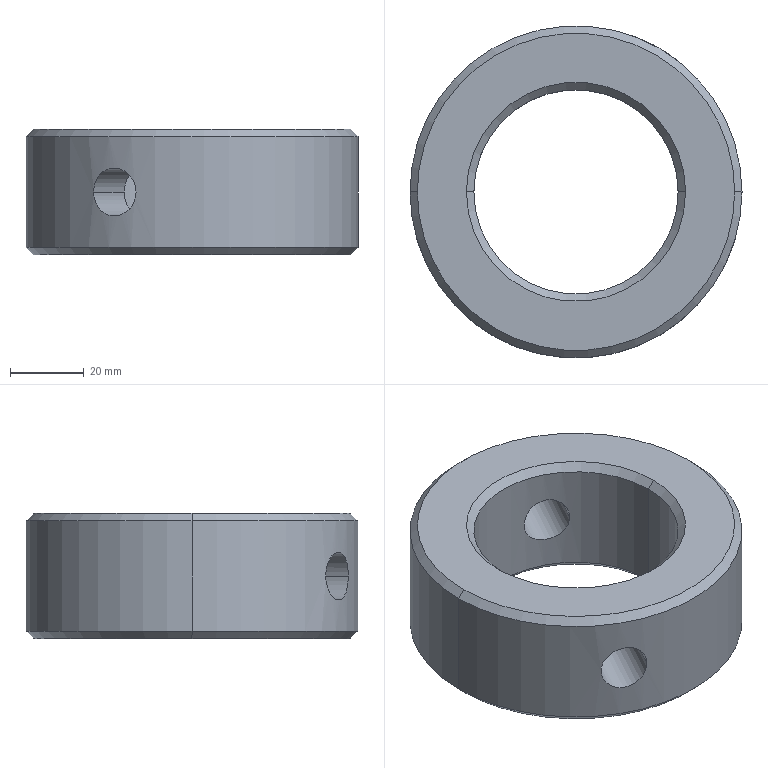Part | SolidWorks | features 3DProfileFeature 1, Chamfer 1, Extrusion 1, HoleWzd 1 | 1 solid | 18 faces | box 90 x 90 x 34 mm | volume 127902 mm3 | cone 8 | cylinder 8 | plane 2 | commonest cylinder face diameters 13 x4 55.4 x2 90 x2
STEP:
#1=CARTESIAN_POINT('',(43.,0.,34.));
#2=VERTEX_POINT('',#1);
#3=CARTESIAN_POINT('',(-43.,0.,34.));
#4=VERTEX_POINT('',#3);
#5=CARTESIAN_POINT('',(0.,0.,34.));
#6=DIRECTION('',(0.,0.,1.));
#7=DIRECTION('',(1.,0.,0.));
#8=AXIS2_PLACEMENT_3D('',#5,#6,#7);
#9=CIRCLE('',#8,43.);
#10=EDGE_CURVE('',#2,#4,#9,.T.);
#11=ORIENTED_EDGE('',*,*,#10,.F.);
#12=CARTESIAN_POINT('',(45.,0.,32.));
#13=VERTEX_POINT('',#12);
#14=CARTESIAN_POINT('',(43.,0.,34.));
#15=DIRECTION('',(0.7071,0.,-0.7071));
#16=VECTOR('',#15,1000.);
#17=LINE('',#14,#16);
#18=EDGE_CURVE('',#2,#13,#17,.T.);
#19=ORIENTED_EDGE('',*,*,#18,.T.);
#20=CARTESIAN_POINT('',(-45.,0.,32.));
#21=VERTEX_POINT('',#20);
#22=CARTESIAN_POINT('',(0.,0.,32.));
#23=DIRECTION('',(0.,0.,-1.));
#24=DIRECTION('',(1.,0.,0.));
#25=AXIS2_PLACEMENT_3D('',#22,#23,#24);
#26=CIRCLE('',#25,45.);
#27=EDGE_CURVE('',#21,#13,#26,.T.);
#28=ORIENTED_EDGE('',*,*,#27,.F.);
#29=CARTESIAN_POINT('',(-43.,0.,34.));
#30=DIRECTION('',(-0.7071,0.,-0.7071));
#31=VECTOR('',#30,1000.);
#32=LINE('',#29,#31);
#33=EDGE_CURVE('',#4,#21,#32,.T.);
#34=ORIENTED_EDGE('',*,*,#33,.F.);
#35=EDGE_LOOP('',(#11,#19,#28,#34));
#36=FACE_OUTER_BOUND('',#35,.T.);
#37=CARTESIAN_POINT('',(0.,0.,34.));
#38=DIRECTION('',(0.,0.,-1.));
#39=DIRECTION('',(-1.,0.,0.));
#40=AXIS2_PLACEMENT_3D('',#37,#38,#39);
#41=CONICAL_SURFACE('',#40,43.,0.7854);
#42=ADVANCED_FACE('',(#36),#41,.T.);
#43=CARTESIAN_POINT('',(-27.7,0.,32.));
#44=VERTEX_POINT('',#43);
#45=CARTESIAN_POINT('',(27.7,0.,32.));
#46=VERTEX_POINT('',#45);
#47=CARTESIAN_POINT('',(0.,0.,32.));
#48=DIRECTION('',(0.,0.,1.));
#49=DIRECTION('',(1.,0.,0.));
#50=AXIS2_PLACEMENT_3D('',#47,#48,#49);
#51=CIRCLE('',#50,27.7);
#52=EDGE_CURVE('',#44,#46,#51,.T.);
#53=ORIENTED_EDGE('',*,*,#52,.F.);
#54=CARTESIAN_POINT('',(-29.7,0.,34.));
#55=VERTEX_POINT('',#54);
#56=CARTESIAN_POINT('',(-27.7,0.,32.));
#57=DIRECTION('',(-0.7071,0.,0.7071));
#58=VECTOR('',#57,1000.);
#59=LINE('',#56,#58);
#60=EDGE_CURVE('',#44,#55,#59,.T.);
#61=ORIENTED_EDGE('',*,*,#60,.T.);
#62=CARTESIAN_POINT('',(29.7,0.,34.));
#63=VERTEX_POINT('',#62);
#64=CARTESIAN_POINT('',(0.,0.,34.));
#65=DIRECTION('',(0.,0.,-1.));
#66=DIRECTION('',(1.,0.,0.));
#67=AXIS2_PLACEMENT_3D('',#64,#65,#66);
#68=CIRCLE('',#67,29.7);
#69=EDGE_CURVE('',#63,#55,#68,.T.);
#70=ORIENTED_EDGE('',*,*,#69,.F.);
#71=CARTESIAN_POINT('',(27.7,0.,32.));
#72=DIRECTION('',(0.7071,0.,0.7071));
#73=VECTOR('',#72,1000.);
#74=LINE('',#71,#73);
#75=EDGE_CURVE('',#46,#63,#74,.T.);
#76=ORIENTED_EDGE('',*,*,#75,.F.);
#77=EDGE_LOOP('',(#53,#61,#70,#76));
#78=FACE_OUTER_BOUND('',#77,.T.);
#79=CARTESIAN_POINT('',(0.,0.,32.));
#80=DIRECTION('',(0.,0.,1.));
#81=DIRECTION('',(1.,0.,0.));
#82=AXIS2_PLACEMENT_3D('',#79,#80,#81);
#83=CONICAL_SURFACE('',#82,27.7,0.7854);
#84=ADVANCED_FACE('',(#78),#83,.F.);
#85=CARTESIAN_POINT('',(27.7,0.,2.));
#86=VERTEX_POINT('',#85);
#87=CARTESIAN_POINT('',(-27.7,0.,2.));
#88=VERTEX_POINT('',#87);
#89=CARTESIAN_POINT('',(0.,0.,2.));
#90=DIRECTION('',(0.,0.,-1.));
#91=DIRECTION('',(1.,0.,0.));
#92=AXIS2_PLACEMENT_3D('',#89,#90,#91);
#93=CIRCLE('',#92,27.7);
#94=EDGE_CURVE('',#86,#88,#93,.T.);
#95=ORIENTED_EDGE('',*,*,#94,.F.);
#96=CARTESIAN_POINT('',(29.7,0.,0.));
#97=VERTEX_POINT('',#96);
#98=CARTESIAN_POINT('',(29.7,0.,0.));
#99=DIRECTION('',(0.7071,0.,-0.7071));
#100=VECTOR('',#99,1000.);
#101=LINE('',#98,#100);
#102=EDGE_CURVE('',#86,#97,#101,.T.);
#103=ORIENTED_EDGE('',*,*,#102,.T.);
#104=CARTESIAN_POINT('',(-29.7,0.,0.));
#105=VERTEX_POINT('',#104);
#106=CARTESIAN_POINT('',(0.,0.,0.));
#107=DIRECTION('',(0.,0.,1.));
#108=DIRECTION('',(1.,0.,0.));
#109=AXIS2_PLACEMENT_3D('',#106,#107,#108);
#110=CIRCLE('',#109,29.7);
#111=EDGE_CURVE('',#105,#97,#110,.T.);
#112=ORIENTED_EDGE('',*,*,#111,.F.);
#113=CARTESIAN_POINT('',(-29.7,0.,0.));
#114=DIRECTION('',(-0.7071,0.,-0.7071));
#115=VECTOR('',#114,1000.);
#116=LINE('',#113,#115);
#117=EDGE_CURVE('',#88,#105,#116,.T.);
#118=ORIENTED_EDGE('',*,*,#117,.F.);
#119=EDGE_LOOP('',(#95,#103,#112,#118));
#120=FACE_OUTER_BOUND('',#119,.T.);
#121=CARTESIAN_POINT('',(0.,0.,0.));
#122=DIRECTION('',(0.,0.,-1.));
#123=DIRECTION('',(-1.,0.,0.));
#124=AXIS2_PLACEMENT_3D('',#121,#122,#123);
#125=CONICAL_SURFACE('',#124,29.7,0.7854);
#126=ADVANCED_FACE('',(#120),#125,.F.);
#127=CARTESIAN_POINT('',(-43.,0.,0.));
#128=VERTEX_POINT('',#127);
#129=CARTESIAN_POINT('',(43.,0.,0.));
#130=VERTEX_POINT('',#129);
#131=CARTESIAN_POINT('',(0.,0.,0.));
#132=DIRECTION('',(0.,0.,-1.));
#133=DIRECTION('',(1.,0.,0.));
#134=AXIS2_PLACEMENT_3D('',#131,#132,#133);
#135=CIRCLE('',#134,43.);
#136=EDGE_CURVE('',#128,#130,#135,.T.);
#137=ORIENTED_EDGE('',*,*,#136,.F.);
#138=CARTESIAN_POINT('',(-45.,0.,2.));
#139=VERTEX_POINT('',#138);
#140=CARTESIAN_POINT('',(-45.,0.,2.));
#141=DIRECTION('',(-0.7071,0.,0.7071));
#142=VECTOR('',#141,1000.);
#143=LINE('',#140,#142);
#144=EDGE_CURVE('',#128,#139,#143,.T.);
#145=ORIENTED_EDGE('',*,*,#144,.T.);
#146=CARTESIAN_POINT('',(45.,0.,2.));
#147=VERTEX_POINT('',#146);
#148=CARTESIAN_POINT('',(0.,0.,2.));
#149=DIRECTION('',(0.,0.,1.));
#150=DIRECTION('',(1.,0.,0.));
#151=AXIS2_PLACEMENT_3D('',#148,#149,#150);
#152=CIRCLE('',#151,45.);
#153=EDGE_CURVE('',#147,#139,#152,.T.);
#154=ORIENTED_EDGE('',*,*,#153,.F.);
#155=CARTESIAN_POINT('',(45.,0.,2.));
#156=DIRECTION('',(0.7071,0.,0.7071));
#157=VECTOR('',#156,1000.);
#158=LINE('',#155,#157);
#159=EDGE_CURVE('',#130,#147,#158,.T.);
#160=ORIENTED_EDGE('',*,*,#159,.F.);
#161=EDGE_LOOP('',(#137,#145,#154,#160));
#162=FACE_OUTER_BOUND('',#161,.T.);
#163=CARTESIAN_POINT('',(0.,0.,2.));
#164=DIRECTION('',(0.,0.,1.));
#165=DIRECTION('',(1.,0.,0.));
#166=AXIS2_PLACEMENT_3D('',#163,#164,#165);
#167=CONICAL_SURFACE('',#166,45.,0.7854);
#168=ADVANCED_FACE('',(#162),#167,.T.);
#169=CARTESIAN_POINT('',(-15.171,-42.366,17.));
#170=VERTEX_POINT('',#169);
#171=CARTESIAN_POINT('',(-26.648,-36.261,17.));
#172=VERTEX_POINT('',#171);
#173=CARTESIAN_POINT('',(-15.171,-42.366,17.));
#174=CARTESIAN_POINT('',(-15.171,-42.366,16.576));
#175=CARTESIAN_POINT('',(-15.21,-42.352,16.153));
#176=CARTESIAN_POINT('',(-15.329,-42.309,15.523));
#177=CARTESIAN_POINT('',(-15.378,-42.291,15.315));
#178=CARTESIAN_POINT('',(-15.496,-42.248,14.908));
#179=CARTESIAN_POINT('',(-15.631,-42.198,14.509));
#180=CARTESIAN_POINT('',(-15.802,-42.134,14.126));
#181=CARTESIAN_POINT('',(-15.991,-42.063,13.75));
#182=CARTESIAN_POINT('',(-16.095,-42.023,13.566));
#183=CARTESIAN_POINT('',(-16.43,-41.894,13.034));
#184=CARTESIAN_POINT('',(-16.681,-41.795,12.707));
#185=CARTESIAN_POINT('',(-17.239,-41.568,12.107));
#186=CARTESIAN_POINT('',(-17.548,-41.439,11.833));
#187=CARTESIAN_POINT('',(-18.197,-41.158,11.361));
#188=CARTESIAN_POINT('',(-18.539,-41.006,11.161));
#189=CARTESIAN_POINT('',(-19.075,-40.758,10.916));
#190=CARTESIAN_POINT('',(-19.259,-40.671,10.843));
#191=CARTESIAN_POINT('',(-19.627,-40.495,10.719));
#192=CARTESIAN_POINT('',(-19.813,-40.404,10.667));
#193=CARTESIAN_POINT('',(-20.371,-40.127,10.543));
#194=CARTESIAN_POINT('',(-20.748,-39.934,10.5));
#195=CARTESIAN_POINT('',(-21.507,-39.53,10.5));
#196=CARTESIAN_POINT('',(-21.877,-39.327,10.542));
#197=CARTESIAN_POINT('',(-22.419,-39.018,10.665));
#198=CARTESIAN_POINT('',(-22.598,-38.915,10.717));
#199=CARTESIAN_POINT('',(-22.951,-38.708,10.84));
#200=CARTESIAN_POINT('',(-23.125,-38.604,10.913));
#201=CARTESIAN_POINT('',(-23.631,-38.298,11.157));
#202=CARTESIAN_POINT('',(-23.948,-38.1,11.357));
#203=CARTESIAN_POINT('',(-24.546,-37.718,11.828));
#204=CARTESIAN_POINT('',(-24.826,-37.533,12.102));
#205=CARTESIAN_POINT('',(-25.326,-37.198,12.7));
#206=CARTESIAN_POINT('',(-25.549,-37.045,13.026));
#207=CARTESIAN_POINT('',(-25.942,-36.77,13.737));
#208=CARTESIAN_POINT('',(-26.108,-36.652,14.113));
#209=CARTESIAN_POINT('',(-26.308,-36.509,14.7));
#210=CARTESIAN_POINT('',(-26.367,-36.467,14.899));
#211=CARTESIAN_POINT('',(-26.468,-36.393,15.306));
#212=CARTESIAN_POINT('',(-26.511,-36.362,15.515));
#213=CARTESIAN_POINT('',(-26.614,-36.286,16.145));
#214=CARTESIAN_POINT('',(-26.648,-36.261,16.57));
#215=CARTESIAN_POINT('',(-26.648,-36.261,17.));
#216=B_SPLINE_CURVE_WITH_KNOTS('',3,(#173,#174,#175,#176,#177,#178,#179,#180,#181,#182,#183,#184,#185,#186,#187,#188,#189,#190,#191,#192,#193,#194,#195,#196,#197,#198,#199,#200,#201,#202,#203,#204,#205,#206,#207,#208,#209,#210,#211,#212,#213,#214,#215),.UNSPECIFIED.,.F.,.F.,(4,2,2,1,2,2,2,2,2,2,2,2,2,2,2,2,2,2,2,2,2,4),(0.02035,0.02162,0.02226,0.02289,0.02353,0.02416,0.02543,0.02671,0.02798,0.02861,0.02925,0.03052,0.03179,0.03243,0.03306,0.03433,0.03561,0.03688,0.03815,0.03878,0.03942,0.04069),.UNSPECIFIED.);
#217=EDGE_CURVE('',#170,#172,#216,.T.);
#218=ORIENTED_EDGE('',*,*,#217,.F.);
#219=CARTESIAN_POINT('',(-6.905,-26.825,17.));
#220=VERTEX_POINT('',#219);
#221=CARTESIAN_POINT('',(26.87,36.678,17.));
#222=DIRECTION('',(0.4696,0.8829,0.));
#223=VECTOR('',#222,1000.);
#224=LINE('',#221,#223);
#225=EDGE_CURVE('',#170,#220,#224,.T.);
#226=ORIENTED_EDGE('',*,*,#225,.T.);
#227=CARTESIAN_POINT('',(-18.383,-20.721,17.));
#228=VERTEX_POINT('',#227);
#229=CARTESIAN_POINT('',(-6.905,-26.825,17.));
#230=CARTESIAN_POINT('',(-6.905,-26.825,16.575));
#231=CARTESIAN_POINT('',(-6.947,-26.815,16.152));
#232=CARTESIAN_POINT('',(-7.114,-26.771,15.308));
#233=CARTESIAN_POINT('',(-7.237,-26.738,14.901));
#234=CARTESIAN_POINT('',(-7.477,-26.672,14.314));
#235=CARTESIAN_POINT('',(-7.567,-26.647,14.122));
#236=CARTESIAN_POINT('',(-7.764,-26.59,13.746));
#237=CARTESIAN_POINT('',(-7.873,-26.558,13.562));
#238=CARTESIAN_POINT('',(-8.219,-26.454,13.032));
#239=CARTESIAN_POINT('',(-8.479,-26.372,12.706));
#240=CARTESIAN_POINT('',(-9.055,-26.18,12.106));
#241=CARTESIAN_POINT('',(-9.373,-26.069,11.833));
#242=CARTESIAN_POINT('',(-10.036,-25.82,11.363));
#243=CARTESIAN_POINT('',(-10.385,-25.683,11.163));
#244=CARTESIAN_POINT('',(-10.933,-25.452,10.916));
#245=CARTESIAN_POINT('',(-11.12,-25.371,10.844));
#246=CARTESIAN_POINT('',(-11.492,-25.204,10.72));
#247=CARTESIAN_POINT('',(-11.867,-25.032,10.616));
#248=CARTESIAN_POINT('',(-12.245,-24.848,10.553));
#249=CARTESIAN_POINT('',(-12.624,-24.657,10.511));
#250=CARTESIAN_POINT('',(-12.816,-24.558,10.5));
#251=CARTESIAN_POINT('',(-13.384,-24.256,10.5));
#252=CARTESIAN_POINT('',(-13.753,-24.049,10.542));
#253=CARTESIAN_POINT('',(-14.471,-23.623,10.707));
#254=CARTESIAN_POINT('',(-14.824,-23.403,10.833));
#255=CARTESIAN_POINT('',(-15.483,-22.972,11.159));
#256=CARTESIAN_POINT('',(-15.793,-22.76,11.358));
#257=CARTESIAN_POINT('',(-16.229,-22.448,11.713));
#258=CARTESIAN_POINT('',(-16.37,-22.346,11.841));
#259=CARTESIAN_POINT('',(-16.637,-22.148,12.11));
#260=CARTESIAN_POINT('',(-16.763,-22.053,12.252));
#261=CARTESIAN_POINT('',(-17.123,-21.776,12.7));
#262=CARTESIAN_POINT('',(-17.338,-21.604,13.028));
#263=CARTESIAN_POINT('',(-17.713,-21.297,13.738));
#264=CARTESIAN_POINT('',(-17.87,-21.166,14.111));
#265=CARTESIAN_POINT('',(-18.06,-21.003,14.697));
#266=CARTESIAN_POINT('',(-18.116,-20.955,14.897));
#267=CARTESIAN_POINT('',(-18.213,-20.871,15.307));
#268=CARTESIAN_POINT('',(-18.253,-20.835,15.516));
#269=CARTESIAN_POINT('',(-18.35,-20.75,16.144));
#270=CARTESIAN_POINT('',(-18.383,-20.721,16.569));
#271=CARTESIAN_POINT('',(-18.383,-20.721,17.));
#272=B_SPLINE_CURVE_WITH_KNOTS('',3,(#229,#230,#231,#232,#233,#234,#235,#236,#237,#238,#239,#240,#241,#242,#243,#244,#245,#246,#247,#248,#249,#250,#251,#252,#253,#254,#255,#256,#257,#258,#259,#260,#261,#262,#263,#264,#265,#266,#267,#268,#269,#270,#271),.UNSPECIFIED.,.F.,.F.,(4,2,2,2,2,2,2,2,2,1,2,2,2,2,2,2,2,2,2,2,2,4),(0.02039,0.02167,0.02294,0.02358,0.02422,0.02549,0.02676,0.02804,0.02868,0.02931,0.02995,0.03059,0.03186,0.03314,0.03441,0.03505,0.03568,0.03696,0.03823,0.03887,0.03951,0.04078),.UNSPECIFIED.);
#273=EDGE_CURVE('',#220,#228,#272,.T.);
#274=ORIENTED_EDGE('',*,*,#273,.T.);
#275=CARTESIAN_POINT('',(15.392,42.782,17.));
#276=DIRECTION('',(0.4696,0.8829,0.));
#277=VECTOR('',#276,1000.);
#278=LINE('',#275,#277);
#279=EDGE_CURVE('',#172,#228,#278,.T.);
#280=ORIENTED_EDGE('',*,*,#279,.F.);
#281=EDGE_LOOP('',(#218,#226,#274,#280));
#282=FACE_OUTER_BOUND('',#281,.T.);
#283=CARTESIAN_POINT('',(21.131,39.73,17.));
#284=DIRECTION('',(0.4696,0.8829,0.));
#285=DIRECTION('',(-0.8829,0.4696,0.));
#286=AXIS2_PLACEMENT_3D('',#283,#284,#285);
#287=CYLINDRICAL_SURFACE('',#286,6.5);
#288=ADVANCED_FACE('',(#282),#287,.F.);
#289=CARTESIAN_POINT('',(6.905,26.825,17.));
#290=VERTEX_POINT('',#289);
#291=CARTESIAN_POINT('',(18.383,20.721,17.));
#292=VERTEX_POINT('',#291);
#293=CARTESIAN_POINT('',(6.905,26.825,17.));
#294=CARTESIAN_POINT('',(6.905,26.825,16.569));
#295=CARTESIAN_POINT('',(6.948,26.815,16.145));
#296=CARTESIAN_POINT('',(7.072,26.782,15.521));
#297=CARTESIAN_POINT('',(7.123,26.769,15.314));
#298=CARTESIAN_POINT('',(7.246,26.736,14.905));
#299=CARTESIAN_POINT('',(7.318,26.716,14.702));
#300=CARTESIAN_POINT('',(7.56,26.649,14.112));
#301=CARTESIAN_POINT('',(7.757,26.593,13.74));
#302=CARTESIAN_POINT('',(8.102,26.489,13.211));
#303=CARTESIAN_POINT('',(8.226,26.451,13.038));
#304=CARTESIAN_POINT('',(8.489,26.368,12.709));
#305=CARTESIAN_POINT('',(8.626,26.323,12.552));
#306=CARTESIAN_POINT('',(9.057,26.179,12.104));
#307=CARTESIAN_POINT('',(9.369,26.07,11.836));
#308=CARTESIAN_POINT('',(10.04,25.819,11.36));
#309=CARTESIAN_POINT('',(10.392,25.68,11.159));
#310=CARTESIAN_POINT('',(10.934,25.451,10.916));
#311=CARTESIAN_POINT('',(11.118,25.372,10.844));
#312=CARTESIAN_POINT('',(11.491,25.205,10.72));
#313=CARTESIAN_POINT('',(11.682,25.117,10.667));
#314=CARTESIAN_POINT('',(12.251,24.847,10.542));
#315=CARTESIAN_POINT('',(12.629,24.657,10.5));
#316=CARTESIAN_POINT('',(13.381,24.257,10.5));
#317=CARTESIAN_POINT('',(13.758,24.045,10.542));
#318=CARTESIAN_POINT('',(14.477,23.619,10.709));
#319=CARTESIAN_POINT('',(14.822,23.404,10.833));
#320=CARTESIAN_POINT('',(15.32,23.079,11.078));
#321=CARTESIAN_POINT('',(15.482,22.97,11.17));
#322=CARTESIAN_POINT('',(15.794,22.757,11.371));
#323=CARTESIAN_POINT('',(15.943,22.652,11.48));
#324=CARTESIAN_POINT('',(16.232,22.447,11.715));
#325=CARTESIAN_POINT('',(16.37,22.346,11.841));
#326=CARTESIAN_POINT('',(16.637,22.148,12.11));
#327=CARTESIAN_POINT('',(16.765,22.051,12.254));
#328=CARTESIAN_POINT('',(17.128,21.772,12.706));
#329=CARTESIAN_POINT('',(17.341,21.602,13.033));
#330=CARTESIAN_POINT('',(17.712,21.298,13.736));
#331=CARTESIAN_POINT('',(17.872,21.164,14.117));
#332=CARTESIAN_POINT('',(18.126,20.947,14.902));
#333=CARTESIAN_POINT('',(18.221,20.864,15.307));
#334=CARTESIAN_POINT('',(18.318,20.778,15.934));
#335=CARTESIAN_POINT('',(18.343,20.757,16.148));
#336=CARTESIAN_POINT('',(18.375,20.728,16.575));
#337=CARTESIAN_POINT('',(18.383,20.721,16.787));
#338=CARTESIAN_POINT('',(18.383,20.721,17.));
#339=B_SPLINE_CURVE_WITH_KNOTS('',3,(#293,#294,#295,#296,#297,#298,#299,#300,#301,#302,#303,#304,#305,#306,#307,#308,#309,#310,#311,#312,#313,#314,#315,#316,#317,#318,#319,#320,#321,#322,#323,#324,#325,#326,#327,#328,#329,#330,#331,#332,#333,#334,#335,#336,#337,#338),.UNSPECIFIED.,.F.,.F.,(4,2,2,2,2,2,2,2,2,2,2,2,2,2,2,2,2,2,2,2,2,2,4),(0.,0.001275,0.001912,0.002549,0.003824,0.004461,0.005098,0.006373,0.007647,0.008285,0.008922,0.0102,0.01147,0.01275,0.01338,0.01402,0.01466,0.01529,0.01657,0.01784,0.01912,0.01976,0.02039),.UNSPECIFIED.);
#340=EDGE_CURVE('',#290,#292,#339,.T.);
#341=ORIENTED_EDGE('',*,*,#340,.T.);
#342=CARTESIAN_POINT('',(26.648,36.261,17.));
#343=VERTEX_POINT('',#342);
#344=CARTESIAN_POINT('',(26.87,36.678,17.));
#345=DIRECTION('',(0.4696,0.8829,0.));
#346=VECTOR('',#345,1000.);
#347=LINE('',#344,#346);
#348=EDGE_CURVE('',#292,#343,#347,.T.);
#349=ORIENTED_EDGE('',*,*,#348,.T.);
#350=CARTESIAN_POINT('',(15.171,42.366,17.));
#351=VERTEX_POINT('',#350);
#352=CARTESIAN_POINT('',(15.171,42.366,17.));
#353=CARTESIAN_POINT('',(15.171,42.366,16.57));
#354=CARTESIAN_POINT('',(15.211,42.351,16.147));
#355=CARTESIAN_POINT('',(15.329,42.309,15.523));
#356=CARTESIAN_POINT('',(15.378,42.291,15.317));
#357=CARTESIAN_POINT('',(15.495,42.248,14.909));
#358=CARTESIAN_POINT('',(15.564,42.223,14.706));
#359=CARTESIAN_POINT('',(15.796,42.137,14.115));
#360=CARTESIAN_POINT('',(15.985,42.066,13.742));
#361=CARTESIAN_POINT('',(16.428,41.895,13.036));
#362=CARTESIAN_POINT('',(16.685,41.794,12.702));
#363=CARTESIAN_POINT('',(17.242,41.567,12.104));
#364=CARTESIAN_POINT('',(17.545,41.44,11.835));
#365=CARTESIAN_POINT('',(18.036,41.228,11.478));
#366=CARTESIAN_POINT('',(18.205,41.153,11.368));
#367=CARTESIAN_POINT('',(18.548,41.,11.167));
#368=CARTESIAN_POINT('',(18.897,40.841,10.986));
#369=CARTESIAN_POINT('',(19.259,40.671,10.843));
#370=CARTESIAN_POINT('',(19.626,40.495,10.719));
#371=CARTESIAN_POINT('',(19.814,40.403,10.667));
#372=CARTESIAN_POINT('',(20.379,40.123,10.542));
#373=CARTESIAN_POINT('',(20.754,39.931,10.5));
#374=CARTESIAN_POINT('',(21.504,39.532,10.5));
#375=CARTESIAN_POINT('',(21.882,39.324,10.542));
#376=CARTESIAN_POINT('',(22.607,38.911,10.709));
#377=CARTESIAN_POINT('',(22.957,38.706,10.831));
#378=CARTESIAN_POINT('',(23.463,38.399,11.076));
#379=CARTESIAN_POINT('',(23.63,38.297,11.168));
#380=CARTESIAN_POINT('',(23.949,38.098,11.369));
#381=CARTESIAN_POINT('',(24.104,38.001,11.479));
#382=CARTESIAN_POINT('',(24.55,37.715,11.831));
#383=CARTESIAN_POINT('',(24.825,37.534,12.101));
#384=CARTESIAN_POINT('',(25.331,37.194,12.707));
#385=CARTESIAN_POINT('',(25.554,37.041,13.034));
#386=CARTESIAN_POINT('',(25.845,36.838,13.562));
#387=CARTESIAN_POINT('',(25.935,36.774,13.744));
#388=CARTESIAN_POINT('',(26.101,36.657,14.12));
#389=CARTESIAN_POINT('',(26.177,36.603,14.315));
#390=CARTESIAN_POINT('',(26.377,36.459,14.905));
#391=CARTESIAN_POINT('',(26.478,36.386,15.31));
#392=CARTESIAN_POINT('',(26.614,36.287,16.144));
#393=CARTESIAN_POINT('',(26.648,36.261,16.575));
#394=CARTESIAN_POINT('',(26.648,36.261,17.));
#395=B_SPLINE_CURVE_WITH_KNOTS('',3,(#352,#353,#354,#355,#356,#357,#358,#359,#360,#361,#362,#363,#364,#365,#366,#367,#368,#369,#370,#371,#372,#373,#374,#375,#376,#377,#378,#379,#380,#381,#382,#383,#384,#385,#386,#387,#388,#389,#390,#391,#392,#393,#394),.UNSPECIFIED.,.F.,.F.,(4,2,2,2,2,2,2,2,1,2,2,2,2,2,2,2,2,2,2,2,2,4),(0.,0.001272,0.001908,0.002544,0.003815,0.005087,0.006359,0.006995,0.007631,0.008267,0.008902,0.01017,0.01145,0.01272,0.01335,0.01399,0.01526,0.01653,0.01717,0.0178,0.01908,0.02035),.UNSPECIFIED.);
#396=EDGE_CURVE('',#351,#343,#395,.T.);
#397=ORIENTED_EDGE('',*,*,#396,.F.);
#398=CARTESIAN_POINT('',(15.392,42.782,17.));
#399=DIRECTION('',(0.4696,0.8829,0.));
#400=VECTOR('',#399,1000.);
#401=LINE('',#398,#400);
#402=EDGE_CURVE('',#290,#351,#401,.T.);
#403=ORIENTED_EDGE('',*,*,#402,.F.);
#404=EDGE_LOOP('',(#341,#349,#397,#403));
#405=FACE_OUTER_BOUND('',#404,.T.);
#406=CARTESIAN_POINT('',(21.131,39.73,17.));
#407=DIRECTION('',(0.4696,0.8829,0.));
#408=DIRECTION('',(-0.8829,0.4696,0.));
#409=AXIS2_PLACEMENT_3D('',#406,#407,#408);
#410=CYLINDRICAL_SURFACE('',#409,6.5);
#411=ADVANCED_FACE('',(#405),#410,.F.);
#412=CARTESIAN_POINT('',(-18.383,-20.721,17.));
#413=CARTESIAN_POINT('',(-18.383,-20.721,17.431));
#414=CARTESIAN_POINT('',(-18.35,-20.75,17.855));
#415=CARTESIAN_POINT('',(-18.254,-20.835,18.479));
#416=CARTESIAN_POINT('',(-18.214,-20.87,18.686));
#417=CARTESIAN_POINT('',(-18.118,-20.953,19.095));
#418=CARTESIAN_POINT('',(-18.061,-21.002,19.298));
#419=CARTESIAN_POINT('',(-17.87,-21.165,19.888));
#420=CARTESIAN_POINT('',(-17.714,-21.297,20.26));
#421=CARTESIAN_POINT('',(-17.435,-21.525,20.789));
#422=CARTESIAN_POINT('',(-17.334,-21.607,20.962));
#423=CARTESIAN_POINT('',(-17.118,-21.778,21.291));
#424=CARTESIAN_POINT('',(-17.004,-21.867,21.448));
#425=CARTESIAN_POINT('',(-16.644,-22.144,21.896));
#426=CARTESIAN_POINT('',(-16.379,-22.341,22.164));
#427=CARTESIAN_POINT('',(-15.796,-22.757,22.64));
#428=CARTESIAN_POINT('',(-15.484,-22.971,22.841));
#429=CARTESIAN_POINT('',(-14.991,-23.293,23.084));
#430=CARTESIAN_POINT('',(-14.823,-23.401,23.156));
#431=CARTESIAN_POINT('',(-14.476,-23.617,23.28));
#432=CARTESIAN_POINT('',(-14.297,-23.726,23.333));
#433=CARTESIAN_POINT('',(-13.754,-24.048,23.458));
#434=CARTESIAN_POINT('',(-13.385,-24.255,23.5));
#435=CARTESIAN_POINT('',(-12.634,-24.655,23.5));
#436=CARTESIAN_POINT('',(-12.247,-24.849,23.458));
#437=CARTESIAN_POINT('',(-11.492,-25.207,23.291));
#438=CARTESIAN_POINT('',(-11.121,-25.373,23.167));
#439=CARTESIAN_POINT('',(-10.573,-25.604,22.922));
#440=CARTESIAN_POINT('',(-10.392,-25.677,22.83));
#441=CARTESIAN_POINT('',(-10.041,-25.817,22.629));
#442=CARTESIAN_POINT('',(-9.871,-25.882,22.52));
#443=CARTESIAN_POINT('',(-9.539,-26.006,22.285));
#444=CARTESIAN_POINT('',(-9.378,-26.065,22.159));
#445=CARTESIAN_POINT('',(-9.065,-26.175,21.89));
#446=CARTESIAN_POINT('',(-8.913,-26.227,21.746));
#447=CARTESIAN_POINT('',(-8.478,-26.372,21.294));
#448=CARTESIAN_POINT('',(-8.218,-26.454,20.967));
#449=CARTESIAN_POINT('',(-7.759,-26.592,20.264));
#450=CARTESIAN_POINT('',(-7.558,-26.649,19.883));
#451=CARTESIAN_POINT('',(-7.237,-26.739,19.098));
#452=CARTESIAN_POINT('',(-7.114,-26.771,18.693));
#453=CARTESIAN_POINT('',(-6.989,-26.804,18.066));
#454=CARTESIAN_POINT('',(-6.958,-26.812,17.852));
#455=CARTESIAN_POINT('',(-6.916,-26.823,17.425));
#456=CARTESIAN_POINT('',(-6.905,-26.825,17.213));
#457=CARTESIAN_POINT('',(-6.905,-26.825,17.));
#458=B_SPLINE_CURVE_WITH_KNOTS('',3,(#412,#413,#414,#415,#416,#417,#418,#419,#420,#421,#422,#423,#424,#425,#426,#427,#428,#429,#430,#431,#432,#433,#434,#435,#436,#437,#438,#439,#440,#441,#442,#443,#444,#445,#446,#447,#448,#449,#450,#451,#452,#453,#454,#455,#456,#457),.UNSPECIFIED.,.F.,.F.,(4,2,2,2,2,2,2,2,2,2,2,2,2,2,2,2,2,2,2,2,2,2,4),(0.,0.001275,0.001912,0.002549,0.003824,0.004461,0.005098,0.006373,0.007647,0.008285,0.008922,0.0102,0.01147,0.01275,0.01338,0.01402,0.01466,0.01529,0.01657,0.01784,0.01912,0.01976,0.02039),.UNSPECIFIED.);
#459=EDGE_CURVE('',#228,#220,#458,.T.);
#460=ORIENTED_EDGE('',*,*,#459,.F.);
#461=ORIENTED_EDGE('',*,*,#273,.F.);
#462=EDGE_LOOP('',(#460,#461));
#463=FACE_BOUND('',#462,.T.);
#464=ORIENTED_EDGE('',*,*,#52,.T.);
#465=CARTESIAN_POINT('',(27.7,0.,34.));
#466=DIRECTION('',(0.,0.,-1.));
#467=VECTOR('',#466,1000.);
#468=LINE('',#465,#467);
#469=EDGE_CURVE('',#46,#86,#468,.T.);
#470=ORIENTED_EDGE('',*,*,#469,.T.);
#471=ORIENTED_EDGE('',*,*,#94,.T.);
#472=CARTESIAN_POINT('',(-27.7,0.,34.));
#473=DIRECTION('',(0.,0.,-1.));
#474=VECTOR('',#473,1000.);
#475=LINE('',#472,#474);
#476=EDGE_CURVE('',#44,#88,#475,.T.);
#477=ORIENTED_EDGE('',*,*,#476,.F.);
#478=EDGE_LOOP('',(#464,#470,#471,#477));
#479=FACE_OUTER_BOUND('',#478,.T.);
#480=CARTESIAN_POINT('',(0.,0.,34.));
#481=DIRECTION('',(0.,0.,-1.));
#482=DIRECTION('',(-1.,0.,0.));
#483=AXIS2_PLACEMENT_3D('',#480,#481,#482);
#484=CYLINDRICAL_SURFACE('',#483,27.7);
#485=ADVANCED_FACE('',(#463,#479),#484,.F.);
#486=ORIENTED_EDGE('',*,*,#396,.T.);
#487=CARTESIAN_POINT('',(26.648,36.261,17.));
#488=CARTESIAN_POINT('',(26.648,36.261,17.424));
#489=CARTESIAN_POINT('',(26.615,36.286,17.847));
#490=CARTESIAN_POINT('',(26.513,36.36,18.477));
#491=CARTESIAN_POINT('',(26.47,36.392,18.685));
#492=CARTESIAN_POINT('',(26.369,36.465,19.092));
#493=CARTESIAN_POINT('',(26.252,36.549,19.491));
#494=CARTESIAN_POINT('',(26.103,36.655,19.874));
#495=CARTESIAN_POINT('',(25.938,36.772,20.25));
#496=CARTESIAN_POINT('',(25.847,36.837,20.434));
#497=CARTESIAN_POINT('',(25.554,37.041,20.966));
#498=CARTESIAN_POINT('',(25.331,37.195,21.293));
#499=CARTESIAN_POINT('',(24.831,37.53,21.893));
#500=CARTESIAN_POINT('',(24.551,37.714,22.167));
#501=CARTESIAN_POINT('',(23.955,38.096,22.639));
#502=CARTESIAN_POINT('',(23.638,38.294,22.839));
#503=CARTESIAN_POINT('',(23.132,38.6,23.084));
#504=CARTESIAN_POINT('',(22.958,38.704,23.157));
#505=CARTESIAN_POINT('',(22.605,38.911,23.281));
#506=CARTESIAN_POINT('',(22.427,39.014,23.333));
#507=CARTESIAN_POINT('',(21.885,39.322,23.457));
#508=CARTESIAN_POINT('',(21.514,39.526,23.5));
#509=CARTESIAN_POINT('',(20.756,39.93,23.5));
#510=CARTESIAN_POINT('',(20.38,40.123,23.458));
#511=CARTESIAN_POINT('',(19.821,40.4,23.335));
#512=CARTESIAN_POINT('',(19.635,40.491,23.283));
#513=CARTESIAN_POINT('',(19.266,40.668,23.16));
#514=CARTESIAN_POINT('',(19.082,40.754,23.087));
#515=CARTESIAN_POINT('',(18.546,41.002,22.843));
#516=CARTESIAN_POINT('',(18.204,41.155,22.643));
#517=CARTESIAN_POINT('',(17.554,41.437,22.172));
#518=CARTESIAN_POINT('',(17.244,41.566,21.898));
#519=CARTESIAN_POINT('',(16.687,41.793,21.3));
#520=CARTESIAN_POINT('',(16.435,41.892,20.974));
#521=CARTESIAN_POINT('',(15.987,42.065,20.263));
#522=CARTESIAN_POINT('',(15.797,42.136,19.887));
#523=CARTESIAN_POINT('',(15.567,42.222,19.3));
#524=CARTESIAN_POINT('',(15.498,42.247,19.101));
#525=CARTESIAN_POINT('',(15.381,42.29,18.694));
#526=CARTESIAN_POINT('',(15.331,42.308,18.485));
#527=CARTESIAN_POINT('',(15.211,42.351,17.855));
#528=CARTESIAN_POINT('',(15.171,42.366,17.43));
#529=CARTESIAN_POINT('',(15.171,42.366,17.));
#530=B_SPLINE_CURVE_WITH_KNOTS('',3,(#487,#488,#489,#490,#491,#492,#493,#494,#495,#496,#497,#498,#499,#500,#501,#502,#503,#504,#505,#506,#507,#508,#509,#510,#511,#512,#513,#514,#515,#516,#517,#518,#519,#520,#521,#522,#523,#524,#525,#526,#527,#528,#529),.UNSPECIFIED.,.F.,.F.,(4,2,2,1,2,2,2,2,2,2,2,2,2,2,2,2,2,2,2,2,2,4),(0.02035,0.02162,0.02226,0.02289,0.02353,0.02416,0.02543,0.02671,0.02798,0.02861,0.02925,0.03052,0.03179,0.03243,0.03306,0.03433,0.03561,0.03688,0.03815,0.03878,0.03942,0.04069),.UNSPECIFIED.);
#531=EDGE_CURVE('',#343,#351,#530,.T.);
#532=ORIENTED_EDGE('',*,*,#531,.T.);
#533=EDGE_LOOP('',(#486,#532));
#534=FACE_BOUND('',#533,.T.);
#535=ORIENTED_EDGE('',*,*,#27,.T.);
#536=CARTESIAN_POINT('',(45.,0.,34.));
#537=DIRECTION('',(0.,0.,-1.));
#538=VECTOR('',#537,1000.);
#539=LINE('',#536,#538);
#540=EDGE_CURVE('',#13,#147,#539,.T.);
#541=ORIENTED_EDGE('',*,*,#540,.T.);
#542=ORIENTED_EDGE('',*,*,#153,.T.);
#543=CARTESIAN_POINT('',(-45.,0.,34.));
#544=DIRECTION('',(0.,0.,-1.));
#545=VECTOR('',#544,1000.);
#546=LINE('',#543,#545);
#547=EDGE_CURVE('',#21,#139,#546,.T.);
#548=ORIENTED_EDGE('',*,*,#547,.F.);
#549=EDGE_LOOP('',(#535,#541,#542,#548));
#550=FACE_OUTER_BOUND('',#549,.T.);
#551=CARTESIAN_POINT('',(0.,0.,34.));
#552=DIRECTION('',(0.,0.,-1.));
#553=DIRECTION('',(-1.,0.,0.));
#554=AXIS2_PLACEMENT_3D('',#551,#552,#553);
#555=CYLINDRICAL_SURFACE('',#554,45.);
#556=ADVANCED_FACE('',(#534,#550),#555,.T.);
#557=ORIENTED_EDGE('',*,*,#69,.T.);
#558=CARTESIAN_POINT('',(0.,0.,34.));
#559=DIRECTION('',(0.,0.,-1.));
#560=DIRECTION('',(1.,0.,0.));
#561=AXIS2_PLACEMENT_3D('',#558,#559,#560);
#562=CIRCLE('',#561,29.7);
#563=EDGE_CURVE('',#55,#63,#562,.T.);
#564=ORIENTED_EDGE('',*,*,#563,.T.);
#565=EDGE_LOOP('',(#557,#564));
#566=FACE_BOUND('',#565,.T.);
#567=CARTESIAN_POINT('',(0.,0.,34.));
#568=DIRECTION('',(0.,0.,1.));
#569=DIRECTION('',(1.,0.,0.));
#570=AXIS2_PLACEMENT_3D('',#567,#568,#569);
#571=CIRCLE('',#570,43.);
#572=EDGE_CURVE('',#4,#2,#571,.T.);
#573=ORIENTED_EDGE('',*,*,#572,.T.);
#574=ORIENTED_EDGE('',*,*,#10,.T.);
#575=EDGE_LOOP('',(#573,#574));
#576=FACE_OUTER_BOUND('',#575,.T.);
#577=CARTESIAN_POINT('',(0.,0.,34.));
#578=DIRECTION('',(0.,0.,1.));
#579=DIRECTION('',(1.,0.,0.));
#580=AXIS2_PLACEMENT_3D('',#577,#578,#579);
#581=PLANE('',#580);
#582=ADVANCED_FACE('',(#566,#576),#581,.T.);
#583=CARTESIAN_POINT('',(0.,0.,0.));
#584=DIRECTION('',(0.,0.,-1.));
#585=DIRECTION('',(1.,0.,0.));
#586=AXIS2_PLACEMENT_3D('',#583,#584,#585);
#587=CIRCLE('',#586,43.);
#588=EDGE_CURVE('',#130,#128,#587,.T.);
#589=ORIENTED_EDGE('',*,*,#588,.T.);
#590=ORIENTED_EDGE('',*,*,#136,.T.);
#591=EDGE_LOOP('',(#589,#590));
#592=FACE_OUTER_BOUND('',#591,.T.);
#593=ORIENTED_EDGE('',*,*,#111,.T.);
#594=CARTESIAN_POINT('',(0.,0.,0.));
#595=DIRECTION('',(0.,0.,1.));
#596=DIRECTION('',(1.,0.,0.));
#597=AXIS2_PLACEMENT_3D('',#594,#595,#596);
#598=CIRCLE('',#597,29.7);
#599=EDGE_CURVE('',#97,#105,#598,.T.);
#600=ORIENTED_EDGE('',*,*,#599,.T.);
#601=EDGE_LOOP('',(#593,#600));
#602=FACE_BOUND('',#601,.T.);
#603=CARTESIAN_POINT('',(0.,0.,0.));
#604=DIRECTION('',(0.,0.,1.));
#605=DIRECTION('',(1.,0.,0.));
#606=AXIS2_PLACEMENT_3D('',#603,#604,#605);
#607=PLANE('',#606);
#608=ADVANCED_FACE('',(#592,#602),#607,.F.);
#609=ORIENTED_EDGE('',*,*,#540,.F.);
#610=CARTESIAN_POINT('',(0.,0.,32.));
#611=DIRECTION('',(0.,0.,-1.));
#612=DIRECTION('',(1.,0.,0.));
#613=AXIS2_PLACEMENT_3D('',#610,#611,#612);
#614=CIRCLE('',#613,45.);
#615=EDGE_CURVE('',#13,#21,#614,.T.);
#616=ORIENTED_EDGE('',*,*,#615,.T.);
#617=ORIENTED_EDGE('',*,*,#547,.T.);
#618=CARTESIAN_POINT('',(0.,0.,2.));
#619=DIRECTION('',(0.,0.,1.));
#620=DIRECTION('',(1.,0.,0.));
#621=AXIS2_PLACEMENT_3D('',#618,#619,#620);
#622=CIRCLE('',#621,45.);
#623=EDGE_CURVE('',#139,#147,#622,.T.);
#624=ORIENTED_EDGE('',*,*,#623,.T.);
#625=EDGE_LOOP('',(#609,#616,#617,#624));
#626=FACE_OUTER_BOUND('',#625,.T.);
#627=CARTESIAN_POINT('',(-26.648,-36.261,17.));
#628=CARTESIAN_POINT('',(-26.648,-36.261,17.43));
#629=CARTESIAN_POINT('',(-26.614,-36.286,17.853));
#630=CARTESIAN_POINT('',(-26.513,-36.36,18.477));
#631=CARTESIAN_POINT('',(-26.471,-36.391,18.683));
#632=CARTESIAN_POINT('',(-26.369,-36.465,19.091));
#633=CARTESIAN_POINT('',(-26.31,-36.508,19.294));
#634=CARTESIAN_POINT('',(-26.109,-36.652,19.885));
#635=CARTESIAN_POINT('',(-25.945,-36.768,20.258));
#636=CARTESIAN_POINT('',(-25.555,-37.04,20.964));
#637=CARTESIAN_POINT('',(-25.328,-37.197,21.298));
#638=CARTESIAN_POINT('',(-24.828,-37.532,21.896));
#639=CARTESIAN_POINT('',(-24.553,-37.713,22.165));
#640=CARTESIAN_POINT('',(-24.103,-38.001,22.522));
#641=CARTESIAN_POINT('',(-23.947,-38.1,22.632));
#642=CARTESIAN_POINT('',(-23.628,-38.298,22.833));
#643=CARTESIAN_POINT('',(-23.301,-38.499,23.014));
#644=CARTESIAN_POINT('',(-22.958,-38.704,23.157));
#645=CARTESIAN_POINT('',(-22.606,-38.91,23.281));
#646=CARTESIAN_POINT('',(-22.425,-39.015,23.333));
#647=CARTESIAN_POINT('',(-21.878,-39.326,23.458));
#648=CARTESIAN_POINT('',(-21.508,-39.53,23.5));
#649=CARTESIAN_POINT('',(-20.758,-39.928,23.5));
#650=CARTESIAN_POINT('',(-20.375,-40.125,23.458));
#651=CARTESIAN_POINT('',(-19.627,-40.496,23.291));
#652=CARTESIAN_POINT('',(-19.261,-40.671,23.169));
#653=CARTESIAN_POINT('',(-18.724,-40.92,22.924));
#654=CARTESIAN_POINT('',(-18.546,-41.001,22.832));
#655=CARTESIAN_POINT('',(-18.202,-41.155,22.631));
#656=CARTESIAN_POINT('',(-18.035,-41.228,22.521));
#657=CARTESIAN_POINT('',(-17.55,-41.438,22.169));
#658=CARTESIAN_POINT('',(-17.245,-41.566,21.899));
#659=CARTESIAN_POINT('',(-16.681,-41.795,21.293));
#660=CARTESIAN_POINT('',(-16.429,-41.894,20.966));
#661=CARTESIAN_POINT('',(-16.098,-42.022,20.438));
#662=CARTESIAN_POINT('',(-15.995,-42.062,20.256));
#663=CARTESIAN_POINT('',(-15.805,-42.133,19.88));
#664=CARTESIAN_POINT('',(-15.718,-42.166,19.685));
#665=CARTESIAN_POINT('',(-15.486,-42.252,19.095));
#666=CARTESIAN_POINT('',(-15.369,-42.294,18.69));
#667=CARTESIAN_POINT('',(-15.211,-42.351,17.856));
#668=CARTESIAN_POINT('',(-15.171,-42.366,17.425));
#669=CARTESIAN_POINT('',(-15.171,-42.366,17.));
#670=B_SPLINE_CURVE_WITH_KNOTS('',3,(#627,#628,#629,#630,#631,#632,#633,#634,#635,#636,#637,#638,#639,#640,#641,#642,#643,#644,#645,#646,#647,#648,#649,#650,#651,#652,#653,#654,#655,#656,#657,#658,#659,#660,#661,#662,#663,#664,#665,#666,#667,#668,#669),.UNSPECIFIED.,.F.,.F.,(4,2,2,2,2,2,2,2,1,2,2,2,2,2,2,2,2,2,2,2,2,4),(0.,0.001272,0.001908,0.002544,0.003815,0.005087,0.006359,0.006995,0.007631,0.008267,0.008902,0.01017,0.01145,0.01272,0.01335,0.01399,0.01526,0.01653,0.01717,0.0178,0.01908,0.02035),.UNSPECIFIED.);
#671=EDGE_CURVE('',#172,#170,#670,.T.);
#672=ORIENTED_EDGE('',*,*,#671,.T.);
#673=ORIENTED_EDGE('',*,*,#217,.T.);
#674=EDGE_LOOP('',(#672,#673));
#675=FACE_BOUND('',#674,.T.);
#676=CARTESIAN_POINT('',(0.,0.,34.));
#677=DIRECTION('',(0.,0.,-1.));
#678=DIRECTION('',(-1.,0.,0.));
#679=AXIS2_PLACEMENT_3D('',#676,#677,#678);
#680=CYLINDRICAL_SURFACE('',#679,45.);
#681=ADVANCED_FACE('',(#626,#675),#680,.T.);
#682=ORIENTED_EDGE('',*,*,#469,.F.);
#683=CARTESIAN_POINT('',(0.,0.,32.));
#684=DIRECTION('',(0.,0.,1.));
#685=DIRECTION('',(1.,0.,0.));
#686=AXIS2_PLACEMENT_3D('',#683,#684,#685);
#687=CIRCLE('',#686,27.7);
#688=EDGE_CURVE('',#46,#44,#687,.T.);
#689=ORIENTED_EDGE('',*,*,#688,.T.);
#690=ORIENTED_EDGE('',*,*,#476,.T.);
#691=CARTESIAN_POINT('',(0.,0.,2.));
#692=DIRECTION('',(0.,0.,-1.));
#693=DIRECTION('',(1.,0.,0.));
#694=AXIS2_PLACEMENT_3D('',#691,#692,#693);
#695=CIRCLE('',#694,27.7);
#696=EDGE_CURVE('',#88,#86,#695,.T.);
#697=ORIENTED_EDGE('',*,*,#696,.T.);
#698=EDGE_LOOP('',(#682,#689,#690,#697));
#699=FACE_OUTER_BOUND('',#698,.T.);
#700=ORIENTED_EDGE('',*,*,#340,.F.);
#701=CARTESIAN_POINT('',(18.383,20.721,17.));
#702=CARTESIAN_POINT('',(18.383,20.721,17.425));
#703=CARTESIAN_POINT('',(18.351,20.749,17.848));
#704=CARTESIAN_POINT('',(18.221,20.863,18.692));
#705=CARTESIAN_POINT('',(18.125,20.947,19.099));
#706=CARTESIAN_POINT('',(17.936,21.109,19.686));
#707=CARTESIAN_POINT('',(17.865,21.169,19.878));
#708=CARTESIAN_POINT('',(17.707,21.301,20.254));
#709=CARTESIAN_POINT('',(17.62,21.374,20.438));
#710=CARTESIAN_POINT('',(17.341,21.602,20.968));
#711=CARTESIAN_POINT('',(17.128,21.772,21.294));
#712=CARTESIAN_POINT('',(16.646,22.142,21.894));
#713=CARTESIAN_POINT('',(16.376,22.344,22.167));
#714=CARTESIAN_POINT('',(15.799,22.755,22.637));
#715=CARTESIAN_POINT('',(15.49,22.967,22.837));
#716=CARTESIAN_POINT('',(14.992,23.293,23.084));
#717=CARTESIAN_POINT('',(14.821,23.402,23.156));
#718=CARTESIAN_POINT('',(14.475,23.618,23.28));
#719=CARTESIAN_POINT('',(14.122,23.832,23.384));
#720=CARTESIAN_POINT('',(13.758,24.043,23.447));
#721=CARTESIAN_POINT('',(13.388,24.251,23.489));
#722=CARTESIAN_POINT('',(13.199,24.354,23.5));
#723=CARTESIAN_POINT('',(12.631,24.656,23.5));
#724=CARTESIAN_POINT('',(12.253,24.846,23.458));
#725=CARTESIAN_POINT('',(11.498,25.204,23.293));
#726=CARTESIAN_POINT('',(11.119,25.374,23.167));
#727=CARTESIAN_POINT('',(10.393,25.679,22.841));
#728=CARTESIAN_POINT('',(10.044,25.818,22.642));
#729=CARTESIAN_POINT('',(9.542,26.005,22.287));
#730=CARTESIAN_POINT('',(9.378,26.065,22.159));
#731=CARTESIAN_POINT('',(9.065,26.175,21.89));
#732=CARTESIAN_POINT('',(8.915,26.227,21.748));
#733=CARTESIAN_POINT('',(8.484,26.37,21.3));
#734=CARTESIAN_POINT('',(8.221,26.453,20.972));
#735=CARTESIAN_POINT('',(7.758,26.593,20.262));
#736=CARTESIAN_POINT('',(7.561,26.649,19.889));
#737=CARTESIAN_POINT('',(7.32,26.715,19.303));
#738=CARTESIAN_POINT('',(7.249,26.735,19.103));
#739=CARTESIAN_POINT('',(7.125,26.768,18.693));
#740=CARTESIAN_POINT('',(7.073,26.782,18.484));
#741=CARTESIAN_POINT('',(6.948,26.815,17.856));
#742=CARTESIAN_POINT('',(6.905,26.825,17.431));
#743=CARTESIAN_POINT('',(6.905,26.825,17.));
#744=B_SPLINE_CURVE_WITH_KNOTS('',3,(#701,#702,#703,#704,#705,#706,#707,#708,#709,#710,#711,#712,#713,#714,#715,#716,#717,#718,#719,#720,#721,#722,#723,#724,#725,#726,#727,#728,#729,#730,#731,#732,#733,#734,#735,#736,#737,#738,#739,#740,#741,#742,#743),.UNSPECIFIED.,.F.,.F.,(4,2,2,2,2,2,2,2,2,1,2,2,2,2,2,2,2,2,2,2,2,4),(0.02039,0.02167,0.02294,0.02358,0.02422,0.02549,0.02676,0.02804,0.02868,0.02931,0.02995,0.03059,0.03186,0.03314,0.03441,0.03505,0.03568,0.03696,0.03823,0.03887,0.03951,0.04078),.UNSPECIFIED.);
#745=EDGE_CURVE('',#292,#290,#744,.T.);
#746=ORIENTED_EDGE('',*,*,#745,.F.);
#747=EDGE_LOOP('',(#700,#746));
#748=FACE_BOUND('',#747,.T.);
#749=CARTESIAN_POINT('',(0.,0.,34.));
#750=DIRECTION('',(0.,0.,-1.));
#751=DIRECTION('',(-1.,0.,0.));
#752=AXIS2_PLACEMENT_3D('',#749,#750,#751);
#753=CYLINDRICAL_SURFACE('',#752,27.7);
#754=ADVANCED_FACE('',(#699,#748),#753,.F.);
#755=ORIENTED_EDGE('',*,*,#348,.F.);
#756=ORIENTED_EDGE('',*,*,#745,.T.);
#757=ORIENTED_EDGE('',*,*,#402,.T.);
#758=ORIENTED_EDGE('',*,*,#531,.F.);
#759=EDGE_LOOP('',(#755,#756,#757,#758));
#760=FACE_OUTER_BOUND('',#759,.T.);
#761=CARTESIAN_POINT('',(21.131,39.73,17.));
#762=DIRECTION('',(0.4696,0.8829,0.));
#763=DIRECTION('',(-0.8829,0.4696,0.));
#764=AXIS2_PLACEMENT_3D('',#761,#762,#763);
#765=CYLINDRICAL_SURFACE('',#764,6.5);
#766=ADVANCED_FACE('',(#760),#765,.F.);
#767=ORIENTED_EDGE('',*,*,#225,.F.);
#768=ORIENTED_EDGE('',*,*,#671,.F.);
#769=ORIENTED_EDGE('',*,*,#279,.T.);
#770=ORIENTED_EDGE('',*,*,#459,.T.);
#771=EDGE_LOOP('',(#767,#768,#769,#770));
#772=FACE_OUTER_BOUND('',#771,.T.);
#773=CARTESIAN_POINT('',(21.131,39.73,17.));
#774=DIRECTION('',(0.4696,0.8829,0.));
#775=DIRECTION('',(-0.8829,0.4696,0.));
#776=AXIS2_PLACEMENT_3D('',#773,#774,#775);
#777=CYLINDRICAL_SURFACE('',#776,6.5);
#778=ADVANCED_FACE('',(#772),#777,.F.);
#779=ORIENTED_EDGE('',*,*,#144,.F.);
#780=ORIENTED_EDGE('',*,*,#588,.F.);
#781=ORIENTED_EDGE('',*,*,#159,.T.);
#782=ORIENTED_EDGE('',*,*,#623,.F.);
#783=EDGE_LOOP('',(#779,#780,#781,#782));
#784=FACE_OUTER_BOUND('',#783,.T.);
#785=CARTESIAN_POINT('',(0.,0.,2.));
#786=DIRECTION('',(0.,0.,1.));
#787=DIRECTION('',(1.,0.,0.));
#788=AXIS2_PLACEMENT_3D('',#785,#786,#787);
#789=CONICAL_SURFACE('',#788,45.,0.7854);
#790=ADVANCED_FACE('',(#784),#789,.T.);
#791=ORIENTED_EDGE('',*,*,#102,.F.);
#792=ORIENTED_EDGE('',*,*,#696,.F.);
#793=ORIENTED_EDGE('',*,*,#117,.T.);
#794=ORIENTED_EDGE('',*,*,#599,.F.);
#795=EDGE_LOOP('',(#791,#792,#793,#794));
#796=FACE_OUTER_BOUND('',#795,.T.);
#797=CARTESIAN_POINT('',(0.,0.,0.));
#798=DIRECTION('',(0.,0.,-1.));
#799=DIRECTION('',(-1.,0.,0.));
#800=AXIS2_PLACEMENT_3D('',#797,#798,#799);
#801=CONICAL_SURFACE('',#800,29.7,0.7854);
#802=ADVANCED_FACE('',(#796),#801,.F.);
#803=ORIENTED_EDGE('',*,*,#60,.F.);
#804=ORIENTED_EDGE('',*,*,#688,.F.);
#805=ORIENTED_EDGE('',*,*,#75,.T.);
#806=ORIENTED_EDGE('',*,*,#563,.F.);
#807=EDGE_LOOP('',(#803,#804,#805,#806));
#808=FACE_OUTER_BOUND('',#807,.T.);
#809=CARTESIAN_POINT('',(0.,0.,32.));
#810=DIRECTION('',(0.,0.,1.));
#811=DIRECTION('',(1.,0.,0.));
#812=AXIS2_PLACEMENT_3D('',#809,#810,#811);
#813=CONICAL_SURFACE('',#812,27.7,0.7854);
#814=ADVANCED_FACE('',(#808),#813,.F.);
#815=ORIENTED_EDGE('',*,*,#18,.F.);
#816=ORIENTED_EDGE('',*,*,#572,.F.);
#817=ORIENTED_EDGE('',*,*,#33,.T.);
#818=ORIENTED_EDGE('',*,*,#615,.F.);
#819=EDGE_LOOP('',(#815,#816,#817,#818));
#820=FACE_OUTER_BOUND('',#819,.T.);
#821=CARTESIAN_POINT('',(0.,0.,34.));
#822=DIRECTION('',(0.,0.,-1.));
#823=DIRECTION('',(-1.,0.,0.));
#824=AXIS2_PLACEMENT_3D('',#821,#822,#823);
#825=CONICAL_SURFACE('',#824,43.,0.7854);
#826=ADVANCED_FACE('',(#820),#825,.T.);
#827=CLOSED_SHELL('',(#42,#84,#126,#168,#288,#411,#485,#556,#582,#608,#681,#754,#766,#778,#790,#802,#814,#826));
#828=MANIFOLD_SOLID_BREP('',#827);
#829=CARTESIAN_POINT('',(0.,0.,0.));
#830=DIRECTION('',(0.,0.,1.));
#831=DIRECTION('',(1.,0.,0.));
#832=AXIS2_PLACEMENT_3D('',#829,#830,#831);
#833=(LENGTH_UNIT()NAMED_UNIT(*)SI_UNIT(.MILLI.,.METRE.));
#834=UNCERTAINTY_MEASURE_WITH_UNIT(LENGTH_MEASURE(0.00001),#833,'','');
#835=(NAMED_UNIT(*)PLANE_ANGLE_UNIT()SI_UNIT($,.RADIAN.));
#836=(NAMED_UNIT(*)SI_UNIT($,.STERADIAN.)SOLID_ANGLE_UNIT());
#837=(GEOMETRIC_REPRESENTATION_CONTEXT(3)GLOBAL_UNCERTAINTY_ASSIGNED_CONTEXT((#834))GLOBAL_UNIT_ASSIGNED_CONTEXT((#833,#835,#836))REPRESENTATION_CONTEXT('',''));
#838=ADVANCED_BREP_SHAPE_REPRESENTATION('',(#828,#832),#837);